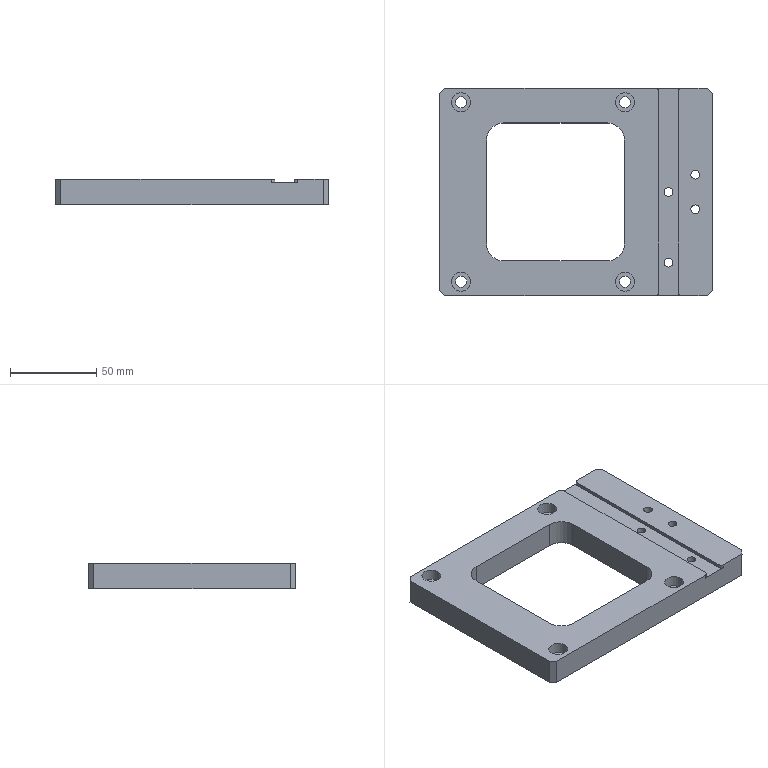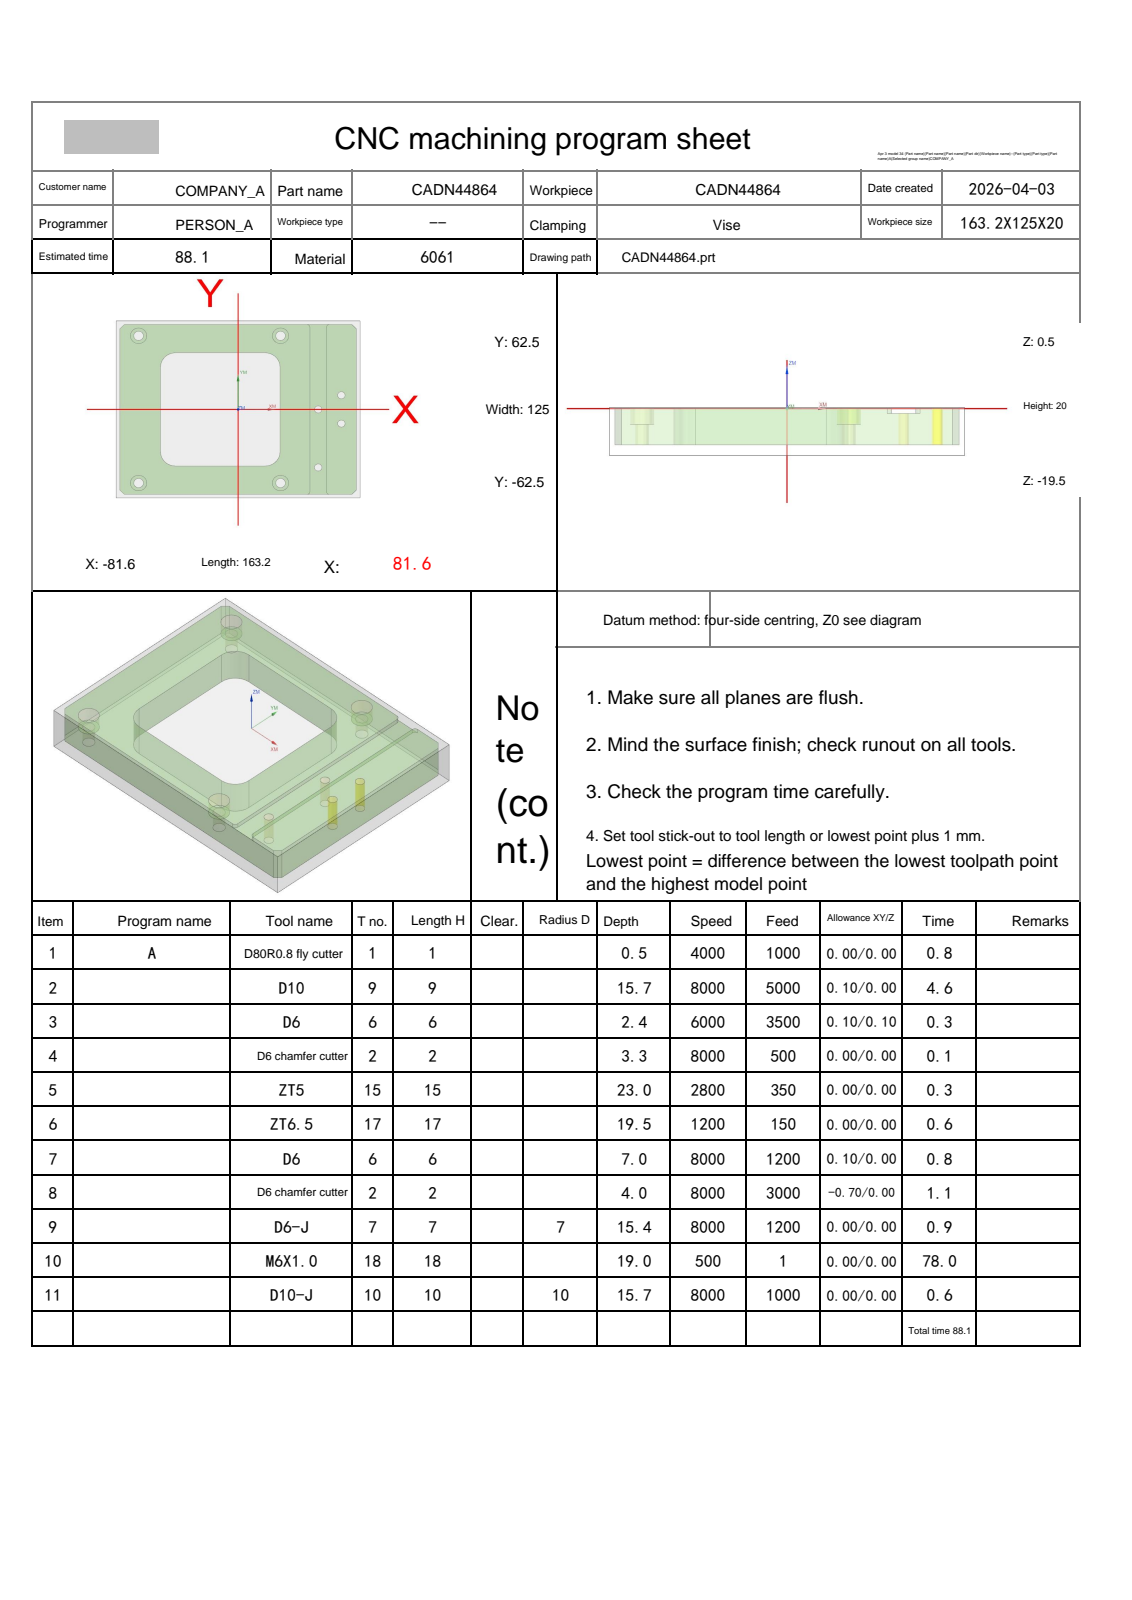NC program | NX | posted by the shop | part box 158.2 x 120 x 15 mm
Lines 961 to 2334 of 2334:
N8 T02 M06
(D6 chamfer cutter  D=6. R=0. H=02 ce=0.00 di=0.00)
G00 G90 G54 X57.022 Y-.25 M03 S8000
G43 H02 Z20.
M08
Z2.099
G01 Z-1.5 F3000.
G03 X57.322 Y-.33 I.3 J.52
X57.842 Y-.03 I0.0 J.6
G01 X57.85 Y0.0
Y58.
G02 X61.15 Y61.3 I3.3 J0.0
G01 X76.1
X76.354 Y61.275
X76.597 Y61.201
X76.822 Y61.081
X77.019 Y60.919
X80.019 Y57.919
X80.181 Y57.722
X80.301 Y57.498
X80.375 Y57.254
X80.4 Y57.
Y-57.
X80.375 Y-57.254
X80.301 Y-57.497
X80.181 Y-57.722
X80.019 Y-57.919
X77.019 Y-60.919
X76.822 Y-61.081
X76.597 Y-61.201
X76.354 Y-61.275
X76.1 Y-61.3
X61.15
G02 X57.85 Y-58. I0.0 J3.3
G01 Y0.0
X57.842 Y.03
G03 X57.322 Y.33 I-.52 J-.3
X57.022 Y.25 I0.0 J-.6
G01 Z2.099
G00 Z20.
X-15.275 Y62.128
Z2.099
G01 Z-1.5
G03 X-15.355 Y61.828 I.52 J-.3
X-15.055 Y61.308 I.6 J0.0
G01 X-15.025 Y61.3
X46.05
G02 X49.35 Y58. I0.0 J-3.3
G01 Y-58.
G02 X46.05 Y-61.3 I-3.3 J0.0
G01 X-76.1
X-76.353 Y-61.275
X-76.597 Y-61.201
X-76.822 Y-61.081
X-77.019 Y-60.919
X-80.019 Y-57.919
X-80.181 Y-57.722
X-80.301 Y-57.497
X-80.375 Y-57.254
X-80.4 Y-57.
Y57.
X-80.375 Y57.254
X-80.301 Y57.497
X-80.181 Y57.722
X-80.019 Y57.919
X-77.019 Y60.919
X-76.822 Y61.081
X-76.597 Y61.201
X-76.354 Y61.275
X-76.1 Y61.3
X-15.025
X-14.995 Y61.308
G03 X-14.695 Y61.828 I-.3 J.52
X-14.775 Y62.128 I-.6 J0.0
G01 Z2.099
G00 Z20.
X-11.65 Y37.872
Z2.099
G01 Z-1.5
G03 X-11.57 Y38.172 I-.52 J.3
X-11.87 Y38.692 I-.6 J0.0
G01 X-11.9 Y38.7
X-41.9
G03 X-50.6 Y30. I0.0 J-8.7
G01 Y-30.
G03 X-41.9 Y-38.7 I8.7 J0.0
G01 X18.1
G03 X26.8 Y-30. I0.0 J8.7
G01 Y30.
G03 X18.1 Y38.7 I-8.7 J0.0
G01 X-11.9
X-11.93 Y38.692
G03 X-12.23 Y38.172 I.3 J-.52
X-12.15 Y37.872 I.6 J0.0
G01 Z2.099
G00 Z20.
X56.976 Y-62.128
Z1.755
G01 Z-3.5
G03 X57.056 Y-61.828 I-.52 J.3
X56.756 Y-61.308 I-.6 J0.0
G01 X56.726 Y-61.3
X50.474
X50.444 Y-61.308
G03 X50.144 Y-61.828 I.3 J-.52
X50.224 Y-62.128 I.6 J0.0
G01 Z1.755
G00 Z20.
Y62.128
Z1.755
G01 Z-3.5
G03 X50.144 Y61.828 I.52 J-.3
X50.444 Y61.308 I.6 J0.0
G01 X50.474 Y61.3
X56.726
X56.756 Y61.308
G03 X57.056 Y61.828 I-.3 J.52
X56.976 Y62.128 I-.6 J0.0
G01 Z1.755
G00 Z20.
G00 G90 X69.257 Y9.216 M03 S8000
Z20.
Z-.5
G01 Z-1. F500.
X69.4 Y8.5
G03 X70.9 Y10. I0.0 J1.5
X69.1 Y11.8 I-1.8 J0.0
X67.3 Y10. I0.0 J-1.8
X69.1 Y8.2 I1.8 J0.0
X70.9 Y10. I0.0 J1.8
X69.4 Y11.5 I-1.5 J0.0
G01 X69.257 Y10.784
Z-.5
G00 Z20.
Y-10.784
Z-.5
G01 Z-1.
X69.4 Y-11.5
G03 X70.9 Y-10. I0.0 J1.5
X69.1 Y-8.2 I-1.8 J0.0
X67.3 Y-10. I0.0 J-1.8
X69.1 Y-11.8 I1.8 J0.0
X70.9 Y-10. I0.0 J1.8
X69.4 Y-8.5 I-1.5 J0.0
G01 X69.257 Y-9.216
Z-.5
G00 Z20.
G00 G90 X-68.609 Y47.643 M03 S8000
Z20.
Z2.5
G01 X-68.434 Y47.561 Z2.43 F800.
X-67.999 Y47.405 Z2.261
X-67.55 Y47.292 Z2.093
X-67.093 Y47.222 Z1.925
X-66.631 Y47.197 Z1.756
X-66.169 Y47.216 Z1.588
X-65.71 Y47.28 Z1.419
X-65.26 Y47.388 Z1.251
X-64.823 Y47.538 Z1.083
X-64.402 Y47.73 Z.914
X-64.001 Y47.961 Z.746
X-63.624 Y48.23 Z.577
X-63.275 Y48.534 Z.409
X-62.957 Y48.87 Z.241
X-62.673 Y49.235 Z.072
X-62.425 Y49.625 Z-.096
X-62.216 Y50.038 Z-.265
X-62.048 Y50.469 Z-.433
X-61.921 Y50.914 Z-.601
X-61.839 Y51.369 Z-.77
X-61.8 Y51.83 Z-.938
Y52. Z-1.
G03 X-66.6 Y56.8 I-4.8 J0.0
X-71.4 Y52. I0.0 J-4.8
X-66.6 Y47.2 I4.8 J0.0
X-61.8 Y52. I0.0 J4.8
X-61.826 Y52.499 I-4.8 J0.0
G01 Z1.5
G00 Z20.
X26.391 Y47.643
Z2.5
G01 X26.566 Y47.561 Z2.43
X27.001 Y47.405 Z2.261
X27.45 Y47.292 Z2.093
X27.907 Y47.222 Z1.925
X28.369 Y47.197 Z1.756
X28.831 Y47.216 Z1.588
X29.29 Y47.28 Z1.419
X29.74 Y47.388 Z1.251
X30.177 Y47.538 Z1.083
X30.598 Y47.73 Z.914
X30.999 Y47.961 Z.746
X31.376 Y48.23 Z.577
X31.725 Y48.534 Z.409
X32.043 Y48.87 Z.241
X32.327 Y49.235 Z.072
X32.575 Y49.625 Z-.096
X32.784 Y50.038 Z-.265
X32.952 Y50.469 Z-.433
X33.079 Y50.914 Z-.601
X33.161 Y51.369 Z-.77
X33.2 Y51.83 Z-.938
Y52. Z-1.
G03 X28.4 Y56.8 I-4.8 J0.0
X23.6 Y52. I0.0 J-4.8
X28.4 Y47.2 I4.8 J0.0
X33.2 Y52. I0.0 J4.8
X33.174 Y52.499 I-4.8 J0.0
G01 Z1.5
G00 Z20.
X26.391 Y-56.357
Z2.5
G01 X26.566 Y-56.439 Z2.43
X27.001 Y-56.595 Z2.261
X27.45 Y-56.708 Z2.093
X27.907 Y-56.778 Z1.925
X28.369 Y-56.803 Z1.756
X28.831 Y-56.784 Z1.588
X29.29 Y-56.72 Z1.419
X29.74 Y-56.612 Z1.251
X30.177 Y-56.462 Z1.083
X30.598 Y-56.27 Z.914
X30.999 Y-56.039 Z.746
X31.376 Y-55.77 Z.577
X31.725 Y-55.466 Z.409
X32.043 Y-55.13 Z.241
X32.327 Y-54.765 Z.072
X32.575 Y-54.375 Z-.096
X32.784 Y-53.962 Z-.265
X32.952 Y-53.531 Z-.433
X33.079 Y-53.086 Z-.601
X33.161 Y-52.631 Z-.77
X33.2 Y-52.17 Z-.938
Y-52. Z-1.
G03 X28.4 Y-47.2 I-4.8 J0.0
X23.6 Y-52. I0.0 J-4.8
X28.4 Y-56.8 I4.8 J0.0
X33.2 Y-52. I0.0 J4.8
X33.174 Y-51.501 I-4.8 J0.0
G01 Z1.5
G00 Z20.
X-68.609 Y-56.357
Z2.5
G01 X-68.434 Y-56.439 Z2.43
X-67.999 Y-56.595 Z2.261
X-67.55 Y-56.708 Z2.093
X-67.093 Y-56.778 Z1.925
X-66.631 Y-56.803 Z1.756
X-66.169 Y-56.784 Z1.588
X-65.71 Y-56.72 Z1.419
X-65.26 Y-56.612 Z1.251
X-64.823 Y-56.462 Z1.083
X-64.402 Y-56.27 Z.914
X-64.001 Y-56.039 Z.746
X-63.624 Y-55.77 Z.577
X-63.275 Y-55.466 Z.409
X-62.957 Y-55.13 Z.241
X-62.673 Y-54.765 Z.072
X-62.425 Y-54.375 Z-.096
X-62.216 Y-53.962 Z-.265
X-62.048 Y-53.531 Z-.433
X-61.921 Y-53.086 Z-.601
X-61.839 Y-52.631 Z-.77
X-61.8 Y-52.17 Z-.938
Y-52. Z-1.
G03 X-66.6 Y-47.2 I-4.8 J0.0
X-71.4 Y-52. I0.0 J-4.8
X-66.6 Y-56.8 I4.8 J0.0
X-61.8 Y-52. I0.0 J4.8
X-61.826 Y-51.501 I-4.8 J0.0
G01 Z1.5
G00 Z20.
G00 G90 X53.4 Y-41.003 M03 S8000
Z20.
Z.5
G01 Y-41.045 Z.499 F500.
X53.461 Y-41.151 Z.494
X53.539 Y-41.196 Z.491
X53.65 Y-41.199 Z.487
X53.747 Y-41.143 Z.483
X53.8 Y-41.045 Z.479
Y-40.955 Z.476
X53.747 Y-40.857 Z.472
X53.65 Y-40.801 Z.469
X53.539 Y-40.804 Z.465
X53.461 Y-40.849 Z.462
X53.4 Y-40.955 Z.457
Y-41.045 Z.454
X53.461 Y-41.151 Z.45
X53.539 Y-41.196 Z.447
X53.65 Y-41.199 Z.443
X53.747 Y-41.143 Z.439
X53.8 Y-41.045 Z.435
Y-40.955 Z.432
X53.747 Y-40.857 Z.428
X53.65 Y-40.801 Z.424
X53.539 Y-40.804 Z.42
X53.461 Y-40.849 Z.417
X53.4 Y-40.955 Z.413
Y-41.045 Z.41
X53.461 Y-41.151 Z.405
X53.539 Y-41.196 Z.402
X53.65 Y-41.199 Z.398
X53.747 Y-41.143 Z.394
X53.8 Y-41.045 Z.391
Y-40.955 Z.387
X53.747 Y-40.857 Z.384
X53.65 Y-40.801 Z.38
X53.539 Y-40.804 Z.376
X53.461 Y-40.849 Z.373
X53.4 Y-40.955 Z.368
Y-41.045 Z.365
X53.461 Y-41.151 Z.361
X53.539 Y-41.196 Z.358
X53.65 Y-41.199 Z.354
X53.747 Y-41.143 Z.35
X53.8 Y-41.045 Z.346
Y-40.955 Z.343
X53.747 Y-40.857 Z.339
X53.65 Y-40.801 Z.335
X53.539 Y-40.804 Z.331
X53.461 Y-40.849 Z.328
X53.4 Y-40.955 Z.324
Y-41.045 Z.321
X53.461 Y-41.151 Z.317
X53.539 Y-41.196 Z.313
X53.65 Y-41.199 Z.309
X53.747 Y-41.143 Z.306
X53.8 Y-41.045 Z.302
Y-40.955 Z.299
X53.747 Y-40.857 Z.295
X53.65 Y-40.801 Z.291
X53.539 Y-40.804 Z.287
X53.461 Y-40.849 Z.284
X53.4 Y-40.955 Z.279
Y-41.045 Z.276
X53.461 Y-41.151 Z.272
X53.539 Y-41.196 Z.269
X53.65 Y-41.199 Z.265
X53.747 Y-41.143 Z.261
X53.8 Y-41.045 Z.257
Y-40.955 Z.254
X53.747 Y-40.857 Z.25
X53.65 Y-40.801 Z.246
X53.539 Y-40.804 Z.242
X53.461 Y-40.849 Z.239
X53.4 Y-40.955 Z.235
Y-41.045 Z.232
X53.461 Y-41.151 Z.228
X53.539 Y-41.196 Z.224
X53.65 Y-41.199 Z.221
X53.747 Y-41.143 Z.217
X53.8 Y-41.045 Z.213
Y-40.955 Z.21
X53.747 Y-40.857 Z.206
X53.65 Y-40.801 Z.202
X53.539 Y-40.804 Z.198
X53.461 Y-40.849 Z.195
X53.4 Y-40.955 Z.191
Y-41.045 Z.187
X53.461 Y-41.151 Z.183
X53.539 Y-41.196 Z.18
X53.65 Y-41.199 Z.176
X53.747 Y-41.143 Z.172
X53.8 Y-41.045 Z.168
Y-40.955 Z.165
X53.747 Y-40.857 Z.161
X53.65 Y-40.801 Z.157
X53.539 Y-40.804 Z.154
X53.461 Y-40.849 Z.15
X53.4 Y-40.955 Z.146
Y-41.045 Z.143
X53.461 Y-41.151 Z.139
X53.539 Y-41.196 Z.136
X53.65 Y-41.199 Z.132
X53.747 Y-41.143 Z.128
X53.8 Y-41.045 Z.124
Y-40.955 Z.121
X53.747 Y-40.857 Z.117
X53.65 Y-40.801 Z.113
X53.539 Y-40.804 Z.109
X53.461 Y-40.849 Z.106
X53.4 Y-40.955 Z.102
Y-41.045 Z.099
X53.461 Y-41.151 Z.094
X53.539 Y-41.196 Z.091
X53.65 Y-41.199 Z.087
X53.747 Y-41.143 Z.083
X53.8 Y-41.045 Z.079
Y-40.955 Z.076
X53.747 Y-40.857 Z.072
X53.65 Y-40.801 Z.069
X53.539 Y-40.804 Z.065
X53.461 Y-40.849 Z.061
X53.4 Y-40.955 Z.057
Y-41.045 Z.054
X53.461 Y-41.151 Z.05
X53.539 Y-41.196 Z.047
X53.65 Y-41.199 Z.043
X53.747 Y-41.143 Z.039
X53.8 Y-41.045 Z.035
Y-40.955 Z.032
X53.747 Y-40.857 Z.028
X53.65 Y-40.801 Z.024
X53.539 Y-40.804 Z.02
X53.461 Y-40.849 Z.017
X53.4 Y-40.955 Z.013
Y-41.045 Z.01
X53.461 Y-41.151 Z.005
X53.539 Y-41.196 Z.002
X53.65 Y-41.199 Z-.002
X53.747 Y-41.143 Z-.006
X53.8 Y-41.045 Z-.009
Y-40.955 Z-.013
X53.747 Y-40.857 Z-.016
X53.65 Y-40.801 Z-.02
X53.539 Y-40.804 Z-.024
X53.461 Y-40.849 Z-.027
X53.4 Y-40.955 Z-.032
Y-41.045 Z-.035
X53.461 Y-41.151 Z-.039
X53.539 Y-41.196 Z-.042
X53.65 Y-41.199 Z-.046
X53.747 Y-41.143 Z-.05
X53.8 Y-41.045 Z-.054
Y-40.955 Z-.057
X53.747 Y-40.857 Z-.061
X53.65 Y-40.801 Z-.065
X53.539 Y-40.804 Z-.069
X53.461 Y-40.849 Z-.072
X53.4 Y-40.955 Z-.076
Y-41.045 Z-.079
X53.461 Y-41.151 Z-.084
X53.539 Y-41.196 Z-.087
X53.65 Y-41.199 Z-.091
X53.747 Y-41.143 Z-.094
X53.8 Y-41.045 Z-.098
Y-40.955 Z-.101
X53.747 Y-40.857 Z-.105
X53.65 Y-40.801 Z-.109
X53.539 Y-40.804 Z-.113
X53.461 Y-40.849 Z-.116
X53.4 Y-40.955 Z-.121
Y-41.045 Z-.124
X53.461 Y-41.151 Z-.128
X53.539 Y-41.196 Z-.131
X53.65 Y-41.199 Z-.135
X53.747 Y-41.143 Z-.139
X53.8 Y-41.045 Z-.143
Y-40.955 Z-.146
X53.747 Y-40.857 Z-.15
X53.65 Y-40.801 Z-.154
X53.539 Y-40.804 Z-.158
X53.461 Y-40.849 Z-.161
X53.4 Y-40.955 Z-.165
Y-41.045 Z-.168
X53.461 Y-41.151 Z-.172
X53.539 Y-41.196 Z-.176
X53.65 Y-41.199 Z-.179
X53.747 Y-41.143 Z-.183
X53.8 Y-41.045 Z-.187
Y-40.955 Z-.19
X53.747 Y-40.857 Z-.194
X53.65 Y-40.801 Z-.198
X53.539 Y-40.804 Z-.202
X53.461 Y-40.849 Z-.205
X53.4 Y-40.955 Z-.209
Y-41.045 Z-.213
X53.461 Y-41.151 Z-.217
X53.539 Y-41.196 Z-.22
X53.65 Y-41.199 Z-.224
X53.747 Y-41.143 Z-.228
X53.8 Y-41.045 Z-.232
Y-40.955 Z-.235
X53.747 Y-40.857 Z-.239
X53.65 Y-40.801 Z-.243
X53.539 Y-40.804 Z-.247
X53.461 Y-40.849 Z-.25
X53.4 Y-40.955 Z-.254
Y-41.045 Z-.257
X53.461 Y-41.151 Z-.261
X53.539 Y-41.196 Z-.264
X53.65 Y-41.199 Z-.268
X53.747 Y-41.143 Z-.272
X53.8 Y-41.045 Z-.276
Y-40.955 Z-.279
X53.747 Y-40.857 Z-.283
X53.65 Y-40.801 Z-.287
X53.539 Y-40.804 Z-.291
X53.461 Y-40.849 Z-.294
X53.4 Y-40.955 Z-.298
Y-41.045 Z-.302
X53.461 Y-41.151 Z-.306
X53.539 Y-41.196 Z-.309
X53.65 Y-41.199 Z-.313
X53.747 Y-41.143 Z-.317
X53.8 Y-41.045 Z-.321
Y-40.955 Z-.324
X53.747 Y-40.857 Z-.328
X53.65 Y-40.801 Z-.332
X53.539 Y-40.804 Z-.335
X53.461 Y-40.849 Z-.339
X53.4 Y-40.955 Z-.343
Y-41.045 Z-.346
X53.461 Y-41.151 Z-.35
X53.539 Y-41.196 Z-.353
X53.65 Y-41.199 Z-.357
X53.747 Y-41.143 Z-.361
X53.8 Y-41.045 Z-.365
Y-40.955 Z-.368
X53.747 Y-40.857 Z-.372
X53.65 Y-40.801 Z-.376
X53.539 Y-40.804 Z-.38
X53.461 Y-40.849 Z-.383
X53.4 Y-40.955 Z-.387
Y-41.045 Z-.39
X53.461 Y-41.151 Z-.395
X53.539 Y-41.196 Z-.398
X53.65 Y-41.199 Z-.402
X53.747 Y-41.143 Z-.406
X53.8 Y-41.045 Z-.409
Y-40.955 Z-.413
X53.747 Y-40.857 Z-.417
X53.65 Y-40.801 Z-.42
X53.539 Y-40.804 Z-.424
X53.461 Y-40.849 Z-.427
X53.4 Y-40.955 Z-.432
Y-41.045 Z-.435
X53.461 Y-41.151 Z-.439
X53.539 Y-41.196 Z-.442
X53.65 Y-41.199 Z-.446
X53.747 Y-41.143 Z-.45
X53.8 Y-41.045 Z-.454
Y-40.955 Z-.457
X53.747 Y-40.857 Z-.461
X53.65 Y-40.801 Z-.465
X53.539 Y-40.804 Z-.469
X53.461 Y-40.849 Z-.472
X53.4 Y-40.955 Z-.476
Y-41.045 Z-.479
X53.461 Y-41.151 Z-.484
X53.539 Y-41.196 Z-.487
X53.65 Y-41.199 Z-.491
X53.747 Y-41.143 Z-.494
X53.8 Y-41.045 Z-.498
Y-40.955 Z-.502
X53.747 Y-40.857 Z-.505
X53.65 Y-40.801 Z-.509
X53.539 Y-40.804 Z-.513
X53.461 Y-40.849 Z-.516
X53.4 Y-40.955 Z-.521
Y-41.045 Z-.524
X53.461 Y-41.151 Z-.528
X53.539 Y-41.196 Z-.531
X53.65 Y-41.199 Z-.535
X53.747 Y-41.143 Z-.539
X53.8 Y-41.045 Z-.543
Y-40.955 Z-.546
X53.747 Y-40.857 Z-.55
X53.65 Y-40.801 Z-.554
X53.539 Y-40.804 Z-.558
X53.461 Y-40.849 Z-.561
X53.4 Y-40.955 Z-.565
Y-41.045 Z-.568
X53.461 Y-41.151 Z-.572
X53.539 Y-41.196 Z-.576
X53.65 Y-41.199 Z-.579
X53.747 Y-41.143 Z-.583
X53.8 Y-41.045 Z-.587
Y-40.955 Z-.59
X53.747 Y-40.857 Z-.594
X53.65 Y-40.801 Z-.598
X53.539 Y-40.804 Z-.602
X53.461 Y-40.849 Z-.605
X53.4 Y-40.955 Z-.609
Y-41.045 Z-.613
X53.461 Y-41.151 Z-.617
X53.539 Y-41.196 Z-.62
X53.65 Y-41.199 Z-.624
X53.747 Y-41.143 Z-.628
X53.8 Y-41.045 Z-.632
Y-40.955 Z-.635
X53.747 Y-40.857 Z-.639
X53.65 Y-40.801 Z-.643
X53.539 Y-40.804 Z-.647
X53.461 Y-40.849 Z-.65
X53.4 Y-40.955 Z-.654
Y-41.045 Z-.657
X53.461 Y-41.151 Z-.661
X53.539 Y-41.196 Z-.664
X53.65 Y-41.199 Z-.668
X53.747 Y-41.143 Z-.672
X53.8 Y-41.045 Z-.676
Y-40.955 Z-.679
X53.747 Y-40.857 Z-.683
X53.65 Y-40.801 Z-.687
X53.539 Y-40.804 Z-.691
X53.461 Y-40.849 Z-.694
X53.4 Y-40.955 Z-.698
Y-41.045 Z-.702
X53.461 Y-41.151 Z-.706
X53.539 Y-41.196 Z-.709
X53.65 Y-41.199 Z-.713
X53.747 Y-41.143 Z-.717
X53.8 Y-41.045 Z-.721
Y-40.955 Z-.724
X53.747 Y-40.857 Z-.728
X53.65 Y-40.801 Z-.732
X53.539 Y-40.804 Z-.735
X53.461 Y-40.849 Z-.739
X53.4 Y-40.955 Z-.743
Y-41.045 Z-.746
X53.461 Y-41.151 Z-.75
X53.539 Y-41.196 Z-.753
X53.65 Y-41.199 Z-.757
X53.747 Y-41.143 Z-.761
X53.8 Y-41.045 Z-.765
Y-40.955 Z-.768
X53.747 Y-40.857 Z-.772
X53.65 Y-40.801 Z-.776
X53.539 Y-40.804 Z-.78
X53.461 Y-40.849 Z-.783
X53.4 Y-40.955 Z-.787
Y-41.045 Z-.79
X53.461 Y-41.151 Z-.795
X53.539 Y-41.196 Z-.798
X53.65 Y-41.199 Z-.802
X53.747 Y-41.143 Z-.806
X53.8 Y-41.045 Z-.81
Y-40.955 Z-.813
X53.747 Y-40.857 Z-.817
X53.65 Y-40.801 Z-.82
X53.539 Y-40.804 Z-.824
X53.461 Y-40.849 Z-.827
X53.4 Y-40.955 Z-.832
Y-41.045 Z-.835
X53.461 Y-41.151 Z-.839
X53.539 Y-41.196 Z-.842
X53.65 Y-41.199 Z-.846
X53.747 Y-41.143 Z-.85
X53.8 Y-41.045 Z-.854
Y-40.955 Z-.857
X53.747 Y-40.857 Z-.861
X53.65 Y-40.801 Z-.865
X53.539 Y-40.804 Z-.869
X53.461 Y-40.849 Z-.872
X53.4 Y-40.955 Z-.876
Y-41.045 Z-.879
X53.461 Y-41.151 Z-.884
X53.539 Y-41.196 Z-.887
X53.65 Y-41.199 Z-.891
X53.747 Y-41.143 Z-.895
X53.8 Y-41.045 Z-.898
Y-40.955 Z-.902
X53.747 Y-40.857 Z-.905
X53.65 Y-40.801 Z-.909
X53.539 Y-40.804 Z-.913
X53.461 Y-40.849 Z-.916
X53.4 Y-40.955 Z-.921
Y-41.045 Z-.924
X53.461 Y-41.151 Z-.928
X53.539 Y-41.196 Z-.931
X53.65 Y-41.199 Z-.935
X53.747 Y-41.143 Z-.939
X53.8 Y-41.045 Z-.943
Y-40.955 Z-.946
X53.747 Y-40.857 Z-.95
X53.65 Y-40.801 Z-.954
X53.539 Y-40.804 Z-.958
X53.461 Y-40.849 Z-.961
X53.4 Y-40.955 Z-.965
Y-41.045 Z-.968
X53.461 Y-41.151 Z-.972
X53.539 Y-41.196 Z-.976
X53.65 Y-41.199 Z-.98
X53.747 Y-41.143 Z-.983
X53.8 Y-41.045 Z-.987
Y-40.955 Z-.99
X53.747 Y-40.857 Z-.994
X53.65 Y-40.801 Z-.998
X53.539 Y-40.804 Z-1.002
X53.461 Y-40.849 Z-1.005
X53.4 Y-40.955 Z-1.01
Y-41.045 Z-1.013
X53.461 Y-41.151 Z-1.017
X53.539 Y-41.196 Z-1.02
X53.65 Y-41.199 Z-1.024
X53.747 Y-41.143 Z-1.028
X53.8 Y-41.045 Z-1.032
Y-40.955 Z-1.035
X53.747 Y-40.857 Z-1.039
X53.65 Y-40.801 Z-1.043
X53.539 Y-40.804 Z-1.047
X53.461 Y-40.849 Z-1.05
X53.4 Y-40.955 Z-1.054
Y-41.045 Z-1.057
X53.461 Y-41.151 Z-1.061
X53.539 Y-41.196 Z-1.065
X53.65 Y-41.199 Z-1.068
X53.747 Y-41.143 Z-1.072
X53.8 Y-41.045 Z-1.076
Y-40.955 Z-1.079
X53.747 Y-40.857 Z-1.083
X53.65 Y-40.801 Z-1.087
X53.539 Y-40.804 Z-1.091
X53.461 Y-40.849 Z-1.094
X53.4 Y-40.955 Z-1.098
Y-41. Z-1.1
G03 X53.6 Y-41.2 I.2 J0.0
X53.8 Y-41. I0.0 J.2
X53.6 Y-40.8 I-.2 J0.0
X53.4 Y-41. I0.0 J-.2
G01 Z-.6
G00 Z20.
X69.509 Y-11.021
Z-.6
G01 Z-1.1
X69.7 Y-11.5
G03 X71.2 Y-10. I0.0 J1.5
X69.1 Y-7.9 I-2.1 J0.0
X67. Y-10. I0.0 J-2.1
X69.1 Y-12.1 I2.1 J0.0
X71.2 Y-10. I0.0 J2.1
X69.7 Y-8.5 I-1.5 J0.0
G01 X69.509 Y-8.979
Z-.6
G00 Z20.
X53.4 Y-.003
Z.5
G01 Y-.045 Z.499
X53.461 Y-.151 Z.494
X53.539 Y-.196 Z.491
X53.65 Y-.199 Z.487
X53.747 Y-.143 Z.483
X53.8 Y-.045 Z.479
Y.045 Z.476
X53.747 Y.143 Z.472
X53.65 Y.199 Z.469
X53.539 Y.196 Z.465
X53.461 Y.151 Z.462
X53.4 Y.045 Z.457
Y-.045 Z.454
X53.461 Y-.151 Z.45
X53.539 Y-.196 Z.447
X53.65 Y-.199 Z.443
X53.747 Y-.143 Z.439
X53.8 Y-.045 Z.435
Y.045 Z.432
X53.747 Y.143 Z.428
X53.65 Y.199 Z.424
X53.539 Y.196 Z.42
X53.461 Y.151 Z.417
X53.4 Y.045 Z.413
Y-.045 Z.41
X53.461 Y-.151 Z.405
X53.539 Y-.196 Z.402
X53.65 Y-.199 Z.398
X53.747 Y-.143 Z.394
X53.8 Y-.045 Z.391
Y.045 Z.387
X53.747 Y.143 Z.384
X53.65 Y.199 Z.38
X53.539 Y.196 Z.376
X53.461 Y.151 Z.373
X53.4 Y.045 Z.368
Y-.045 Z.365
X53.461 Y-.151 Z.361
X53.539 Y-.196 Z.358
X53.65 Y-.199 Z.354
X53.747 Y-.143 Z.35
X53.8 Y-.045 Z.346
Y.045 Z.343
X53.747 Y.143 Z.339
X53.65 Y.199 Z.335
X53.539 Y.196 Z.331
X53.461 Y.151 Z.328
X53.4 Y.045 Z.324
Y-.045 Z.321
X53.461 Y-.151 Z.317
X53.539 Y-.196 Z.313
X53.65 Y-.199 Z.309
X53.747 Y-.143 Z.306
X53.8 Y-.045 Z.302
Y.045 Z.299
X53.747 Y.143 Z.295
X53.65 Y.199 Z.291
X53.539 Y.196 Z.287
X53.461 Y.151 Z.284
X53.4 Y.045 Z.279
Y-.045 Z.276
X53.461 Y-.151 Z.272
X53.539 Y-.196 Z.269
X53.65 Y-.199 Z.265
X53.747 Y-.143 Z.261
X53.8 Y-.045 Z.257
Y.045 Z.254
X53.747 Y.143 Z.25
X53.65 Y.199 Z.246
X53.539 Y.196 Z.242
X53.461 Y.151 Z.239
X53.4 Y.045 Z.235
Y-.045 Z.232
X53.461 Y-.151 Z.228
X53.539 Y-.196 Z.224
X53.65 Y-.199 Z.221
X53.747 Y-.143 Z.217
X53.8 Y-.045 Z.213
Y.045 Z.21
X53.747 Y.143 Z.206
X53.65 Y.199 Z.202
X53.539 Y.196 Z.198
X53.461 Y.151 Z.195
X53.4 Y.045 Z.191
Y-.045 Z.187
X53.461 Y-.151 Z.183
X53.539 Y-.196 Z.18
X53.65 Y-.199 Z.176
X53.747 Y-.143 Z.172
X53.8 Y-.045 Z.168
Y.045 Z.165
X53.747 Y.143 Z.161
X53.65 Y.199 Z.157
X53.539 Y.196 Z.154
X53.461 Y.151 Z.15
X53.4 Y.045 Z.146
Y-.045 Z.143
X53.461 Y-.151 Z.139
X53.539 Y-.196 Z.136
X53.65 Y-.199 Z.132
X53.747 Y-.143 Z.128
X53.8 Y-.045 Z.124
Y.045 Z.121
X53.747 Y.143 Z.117
X53.65 Y.199 Z.113
X53.539 Y.196 Z.109
X53.461 Y.151 Z.106
X53.4 Y.045 Z.102
Y-.045 Z.099
X53.461 Y-.151 Z.094
X53.539 Y-.196 Z.091
X53.65 Y-.199 Z.087
X53.747 Y-.143 Z.083
X53.8 Y-.045 Z.079
Y.045 Z.076
X53.747 Y.143 Z.072
X53.65 Y.199 Z.069
X53.539 Y.196 Z.065
X53.461 Y.151 Z.061
X53.4 Y.045 Z.057
Y-.045 Z.054
X53.461 Y-.151 Z.05
X53.539 Y-.196 Z.047
X53.65 Y-.199 Z.043
X53.747 Y-.143 Z.039
X53.8 Y-.045 Z.035
Y.045 Z.032
X53.747 Y.143 Z.028
X53.65 Y.199 Z.024
X53.539 Y.196 Z.02
X53.461 Y.151 Z.017
X53.4 Y.045 Z.013
Y-.045 Z.01
X53.461 Y-.151 Z.005
X53.539 Y-.196 Z.002
X53.65 Y-.199 Z-.002
X53.747 Y-.143 Z-.006
X53.8 Y-.045 Z-.009
Y.045 Z-.013
X53.747 Y.143 Z-.016
X53.65 Y.199 Z-.02
X53.539 Y.196 Z-.024
X53.461 Y.151 Z-.027
X53.4 Y.045 Z-.032
Y-.045 Z-.035
X53.461 Y-.151 Z-.039
X53.539 Y-.196 Z-.042
X53.65 Y-.199 Z-.046
X53.747 Y-.143 Z-.05
X53.8 Y-.045 Z-.054
Y.045 Z-.057
X53.747 Y.143 Z-.061
X53.65 Y.199 Z-.065
X53.539 Y.196 Z-.069
X53.461 Y.151 Z-.072
X53.4 Y.045 Z-.076
Y-.045 Z-.079
X53.461 Y-.151 Z-.084
X53.539 Y-.196 Z-.087
X53.65 Y-.199 Z-.091
X53.747 Y-.143 Z-.094
X53.8 Y-.045 Z-.098
Y.045 Z-.101
X53.747 Y.143 Z-.105
X53.65 Y.199 Z-.109
X53.539 Y.196 Z-.113
X53.461 Y.151 Z-.116
X53.4 Y.045 Z-.121
Y-.045 Z-.124
X53.461 Y-.151 Z-.128
X53.539 Y-.196 Z-.131
X53.65 Y-.199 Z-.135
X53.747 Y-.143 Z-.139
X53.8 Y-.045 Z-.143
Y.045 Z-.146
X53.747 Y.143 Z-.15
X53.65 Y.199 Z-.154
X53.539 Y.196 Z-.158
X53.461 Y.151 Z-.161
X53.4 Y.045 Z-.165
Y-.045 Z-.168
X53.461 Y-.151 Z-.172
X53.539 Y-.196 Z-.176
X53.65 Y-.199 Z-.179
X53.747 Y-.143 Z-.183
X53.8 Y-.045 Z-.187
Y.045 Z-.19
X53.747 Y.143 Z-.194
X53.65 Y.199 Z-.198
X53.539 Y.196 Z-.202
X53.461 Y.151 Z-.205
X53.4 Y.045 Z-.209
Y-.045 Z-.213
X53.461 Y-.151 Z-.217
X53.539 Y-.196 Z-.22
X53.65 Y-.199 Z-.224
X53.747 Y-.143 Z-.228
X53.8 Y-.045 Z-.232
Y.045 Z-.235
X53.747 Y.143 Z-.239
X53.65 Y.199 Z-.243
X53.539 Y.196 Z-.247
X53.461 Y.151 Z-.25
X53.4 Y.045 Z-.254
Y-.045 Z-.257
X53.461 Y-.151 Z-.261
X53.539 Y-.196 Z-.264
X53.65 Y-.199 Z-.268
X53.747 Y-.143 Z-.272
X53.8 Y-.045 Z-.276
Y.045 Z-.279
X53.747 Y.143 Z-.283
X53.65 Y.199 Z-.287
X53.539 Y.196 Z-.291
X53.461 Y.151 Z-.294
X53.4 Y.045 Z-.298
Y-.045 Z-.302
X53.461 Y-.151 Z-.306
X53.539 Y-.196 Z-.309
X53.65 Y-.199 Z-.313
X53.747 Y-.143 Z-.317
X53.8 Y-.045 Z-.321
Y.045 Z-.324
X53.747 Y.143 Z-.328
X53.65 Y.199 Z-.332
X53.539 Y.196 Z-.335
X53.461 Y.151 Z-.339
X53.4 Y.045 Z-.343
Y-.045 Z-.346
X53.461 Y-.151 Z-.35
X53.539 Y-.196 Z-.353
X53.65 Y-.199 Z-.357
X53.747 Y-.143 Z-.361
X53.8 Y-.045 Z-.365
Y.045 Z-.368
X53.747 Y.143 Z-.372
X53.65 Y.199 Z-.376
X53.539 Y.196 Z-.38
X53.461 Y.151 Z-.383
X53.4 Y.045 Z-.387
Y-.045 Z-.39
X53.461 Y-.151 Z-.395
X53.539 Y-.196 Z-.398
X53.65 Y-.199 Z-.402
X53.747 Y-.143 Z-.406
X53.8 Y-.045 Z-.409
Y.045 Z-.413
X53.747 Y.143 Z-.417
X53.65 Y.199 Z-.42
X53.539 Y.196 Z-.424
X53.461 Y.151 Z-.427
X53.4 Y.045 Z-.432
Y-.045 Z-.435
X53.461 Y-.151 Z-.439
X53.539 Y-.196 Z-.442
X53.65 Y-.199 Z-.446
X53.747 Y-.143 Z-.45
X53.8 Y-.045 Z-.454
Y.045 Z-.457
X53.747 Y.143 Z-.461
X53.65 Y.199 Z-.465
X53.539 Y.196 Z-.469
X53.461 Y.151 Z-.472
X53.4 Y.045 Z-.476
Y-.045 Z-.479
X53.461 Y-.151 Z-.484
X53.539 Y-.196 Z-.487
X53.65 Y-.199 Z-.491
X53.747 Y-.143 Z-.494
X53.8 Y-.045 Z-.498
Y.045 Z-.502
X53.747 Y.143 Z-.505
X53.65 Y.199 Z-.509
X53.539 Y.196 Z-.513
X53.461 Y.151 Z-.516
X53.4 Y.045 Z-.521
Y-.045 Z-.524
X53.461 Y-.151 Z-.528
X53.539 Y-.196 Z-.531
X53.65 Y-.199 Z-.535
X53.747 Y-.143 Z-.539
X53.8 Y-.045 Z-.543
Y.045 Z-.546
X53.747 Y.143 Z-.55
X53.65 Y.199 Z-.554
X53.539 Y.196 Z-.558
X53.461 Y.151 Z-.561
X53.4 Y.045 Z-.565
Y-.045 Z-.568
X53.461 Y-.151 Z-.572
X53.539 Y-.196 Z-.576
X53.65 Y-.199 Z-.579
X53.747 Y-.143 Z-.583
X53.8 Y-.045 Z-.587
Y.045 Z-.59
X53.747 Y.143 Z-.594
X53.65 Y.199 Z-.598
X53.539 Y.196 Z-.602
X53.461 Y.151 Z-.605
X53.4 Y.045 Z-.609
Y-.045 Z-.613
X53.461 Y-.151 Z-.617
X53.539 Y-.196 Z-.62
X53.65 Y-.199 Z-.624
X53.747 Y-.143 Z-.628
X53.8 Y-.045 Z-.632
Y.045 Z-.635
X53.747 Y.143 Z-.639
X53.65 Y.199 Z-.643
X53.539 Y.196 Z-.647
X53.461 Y.151 Z-.65
X53.4 Y.045 Z-.654
Y-.045 Z-.657
X53.461 Y-.151 Z-.661
X53.539 Y-.196 Z-.664
X53.65 Y-.199 Z-.668
X53.747 Y-.143 Z-.672
X53.8 Y-.045 Z-.676
Y.045 Z-.679
X53.747 Y.143 Z-.683
X53.65 Y.199 Z-.687
X53.539 Y.196 Z-.691
X53.461 Y.151 Z-.694
X53.4 Y.045 Z-.698
Y-.045 Z-.702
X53.461 Y-.151 Z-.706
X53.539 Y-.196 Z-.709
X53.65 Y-.199 Z-.713
X53.747 Y-.143 Z-.717
X53.8 Y-.045 Z-.721
Y.045 Z-.724
X53.747 Y.143 Z-.728
X53.65 Y.199 Z-.732
X53.539 Y.196 Z-.735
X53.461 Y.151 Z-.739
X53.4 Y.045 Z-.743
Y-.045 Z-.746
X53.461 Y-.151 Z-.75
X53.539 Y-.196 Z-.753
X53.65 Y-.199 Z-.757
X53.747 Y-.143 Z-.761
X53.8 Y-.045 Z-.765
Y.045 Z-.768
X53.747 Y.143 Z-.772
X53.65 Y.199 Z-.776
X53.539 Y.196 Z-.78
X53.461 Y.151 Z-.783
X53.4 Y.045 Z-.787
Y-.045 Z-.79
X53.461 Y-.151 Z-.795
X53.539 Y-.196 Z-.798
X53.65 Y-.199 Z-.802
X53.747 Y-.143 Z-.806
X53.8 Y-.045 Z-.81
Y.045 Z-.813
X53.747 Y.143 Z-.817
X53.65 Y.199 Z-.82
X53.539 Y.196 Z-.824
X53.461 Y.151 Z-.827
X53.4 Y.045 Z-.832
Y-.045 Z-.835
X53.461 Y-.151 Z-.839
X53.539 Y-.196 Z-.842
X53.65 Y-.199 Z-.846
X53.747 Y-.143 Z-.85
X53.8 Y-.045 Z-.854
Y.045 Z-.857
X53.747 Y.143 Z-.861
X53.65 Y.199 Z-.865
X53.539 Y.196 Z-.869
X53.461 Y.151 Z-.872
X53.4 Y.045 Z-.876
Y-.045 Z-.879
X53.461 Y-.151 Z-.884
X53.539 Y-.196 Z-.887
X53.65 Y-.199 Z-.891
X53.747 Y-.143 Z-.895
X53.8 Y-.045 Z-.898
Y.045 Z-.902
X53.747 Y.143 Z-.905
X53.65 Y.199 Z-.909
X53.539 Y.196 Z-.913
X53.461 Y.151 Z-.916
X53.4 Y.045 Z-.921
Y-.045 Z-.924
X53.461 Y-.151 Z-.928
X53.539 Y-.196 Z-.931
X53.65 Y-.199 Z-.935
X53.747 Y-.143 Z-.939
X53.8 Y-.045 Z-.943
Y.045 Z-.946
X53.747 Y.143 Z-.95
X53.65 Y.199 Z-.954
X53.539 Y.196 Z-.958
X53.461 Y.151 Z-.961
X53.4 Y.045 Z-.965
Y-.045 Z-.968
X53.461 Y-.151 Z-.972
X53.539 Y-.196 Z-.976
X53.65 Y-.199 Z-.98
X53.747 Y-.143 Z-.983
X53.8 Y-.045 Z-.987
Y.045 Z-.99
X53.747 Y.143 Z-.994
X53.65 Y.199 Z-.998
X53.539 Y.196 Z-1.002
X53.461 Y.151 Z-1.005
X53.4 Y.045 Z-1.01
Y-.045 Z-1.013
X53.461 Y-.151 Z-1.017
X53.539 Y-.196 Z-1.02
X53.65 Y-.199 Z-1.024
X53.747 Y-.143 Z-1.028
X53.8 Y-.045 Z-1.032
Y.045 Z-1.035
X53.747 Y.143 Z-1.039
X53.65 Y.199 Z-1.043
X53.539 Y.196 Z-1.047
X53.461 Y.151 Z-1.05
X53.4 Y.045 Z-1.054
Y-.045 Z-1.057
X53.461 Y-.151 Z-1.061
X53.539 Y-.196 Z-1.065
X53.65 Y-.199 Z-1.068
X53.747 Y-.143 Z-1.072
X53.8 Y-.045 Z-1.076
Y.045 Z-1.079
X53.747 Y.143 Z-1.083
X53.65 Y.199 Z-1.087
X53.539 Y.196 Z-1.091
X53.461 Y.151 Z-1.094
X53.4 Y.045 Z-1.098
Y0.0 Z-1.1
G03 X53.6 Y-.2 I.2 J0.0
X53.8 Y0.0 I0.0 J.2
X53.6 Y.2 I-.2 J0.0
X53.4 Y0.0 I0.0 J-.2
G01 Z-.6
G00 Z20.
X69.509 Y8.979
Z-.6
G01 Z-1.1
X69.7 Y8.5
G03 X71.2 Y10. I0.0 J1.5
X69.1 Y12.1 I-2.1 J0.0
X67. Y10. I0.0 J-2.1
X69.1 Y7.9 I2.1 J0.0
X71.2 Y10. I0.0 J2.1
X69.7 Y11.5 I-1.5 J0.0
G01 X69.509 Y11.021
Z-.6
G00 Z20.
G91 G28 Z0.0
M05
M09
G91 G28 Z0.0
M01
N9 T07 M06
(D6-J  D=6. R=0. H=07 ce=0.00 di=0.00)
G00 G90 G54 X28.4 Y52. M03 S8000
G43 H07 Z20.
M08
Z0.0
G41 D07
G01 X28.432 Y51.803 F500.
G03 X29.658 Y50.758 I1.226 J.197
X30.9 Y52. I0.0 J1.242
X30.9 Y52. Z-5. I-2.5 J0.0
X27.627 Y54.378 Z-6.5 I-2.5 J0.0
X25.9 Y52. I.773 J-2.378
X28.4 Y49.5 I2.5 J0.0
X30.9 Y52. I0.0 J2.5
X28.4 Y54.5 I-2.5 J0.0
X27.627 Y54.378 I0.0 J-2.5
X26.769 Y53.196 I.384 J-1.181
X28.011 Y51.954 I1.242 J0.0
G01 X28.202 Y51.969
G40 X28.4 Y52.
G00 Z20.
X-66.6
Z0.0
G41 D07
G01 X-66.568 Y51.803
G03 X-65.342 Y50.758 I1.226 J.197
X-64.1 Y52. I0.0 J1.242
X-64.1 Y52. Z-5. I-2.5 J0.0
X-67.373 Y54.378 Z-6.5 I-2.5 J0.0
X-69.1 Y52. I.773 J-2.378
X-66.6 Y49.5 I2.5 J0.0
X-64.1 Y52. I0.0 J2.5
X-66.6 Y54.5 I-2.5 J0.0
X-67.373 Y54.378 I0.0 J-2.5
X-68.231 Y53.196 I.384 J-1.181
X-66.989 Y51.954 I1.242 J0.0
G01 X-66.798 Y51.969
G40 X-66.6 Y52.
G00 Z20.
G00 G90 X28.4 Y-52. M03 S8000
Z20.
Z0.0
G41 D07
G01 X28.432 Y-52.197 F500.
G03 X29.658 Y-53.242 I1.226 J.197
X30.9 Y-52. I0.0 J1.242
X30.9 Y-52. Z-5. I-2.5 J0.0
X27.627 Y-49.622 Z-6.5 I-2.5 J0.0
X25.9 Y-52. I.773 J-2.378
X28.4 Y-54.5 I2.5 J0.0
X30.9 Y-52. I0.0 J2.5
X28.4 Y-49.5 I-2.5 J0.0
X27.627 Y-49.622 I0.0 J-2.5
X26.769 Y-50.804 I.384 J-1.181
X28.011 Y-52.046 I1.242 J0.0
G01 X28.202 Y-52.031
G40 X28.4 Y-52.
G00 Z20.
X-66.6
Z0.0
G41 D07
G01 X-66.568 Y-52.197
G03 X-65.342 Y-53.242 I1.226 J.197
X-64.1 Y-52. I0.0 J1.242
X-64.1 Y-52. Z-5. I-2.5 J0.0
X-67.373 Y-49.622 Z-6.5 I-2.5 J0.0
X-69.1 Y-52. I.773 J-2.378
X-66.6 Y-54.5 I2.5 J0.0
X-64.1 Y-52. I0.0 J2.5
X-66.6 Y-49.5 I-2.5 J0.0
X-67.373 Y-49.622 I0.0 J-2.5
X-68.231 Y-50.804 I.384 J-1.181
X-66.989 Y-52.046 I1.242 J0.0
G01 X-66.798 Y-52.031
G40 X-66.6 Y-52.
G00 Z20.
G00 G90 X64.85 Y-64.1 M03 S6000
Z20.
Z-1.5
G01 Z-2. F1200.
G41 D07
Y-64.
G03 X63.85 Y-63. I-1. J0.0
G01 X61.15
G02 X56.15 Y-58. I0.0 J5.
G01 Y58.
G02 X61.15 Y63. I5. J0.0
G01 X63.85
G03 X64.85 Y64. I0.0 J1.
G01 G40 Y64.1
Z-1.5
G00 Z20.
X42.35
Z-1.5
G01 Z-2.
G41 D07
Y64.
G03 X43.35 Y63. I1. J0.0
G01 X46.05
G02 X51.05 Y58. I0.0 J-5.
G01 Y-58.
G02 X46.05 Y-63. I-5. J0.0
G01 X43.35
G03 X42.35 Y-64. I0.0 J-1.
G01 G40 Y-64.1
Z-1.5
G00 Z20.
G00 G90 X-42.9 Y-35.816 M03 S6000
Z20.
Z-14.35
G01 Z-14.85 F1000.
G41 D07
Y-36.
G03 X-41.9 Y-37. I1. J0.0
G01 X18.1
G03 X25.1 Y-30. I0.0 J7.
G01 Y30.
G03 X18.1 Y37. I-7. J0.0
G01 X-41.9
G03 X-48.9 Y30. I0.0 J-7.
G01 Y-30.
G03 X-41.9 Y-37. I7. J0.0
G01 X-41.4
G03 X-40.4 Y-36. I0.0 J1.
G01 G40 Y-35.9
Z-14.35
G00 Z20.
G91 G28 Z0.0
M05
M09
G91 G28 Z0.0
M01
N10 T18 M06
(M6X1.0 D=5. DR_a=180 H=18)
G00 G90 G54 X53.6 Y-41. M03 S500
G43 H18 Z20.
M08
G95
G98 G84 X53.6 Y-41. Z-18.5 R1. F1. Q3.
X69.1 Y-10.
Y10.
X53.6 Y0.0
G80
G94
G00 Z20.
G91 G28 Z0.0
M05
M09
G91 G28 Z0.0
M01
N11 T10 M06
(D10-J  D=10. R=0. H=10 ce=0.00 di=0.00)
G00 G90 G54 X-77.113 Y66.116 M03 S8000
G43 H10 Z20.
M08
Z-14.7
G01 Z-15.2 F1000.
G41 D10
X-77.097 Y65.917
G03 X-76.1 Y65. I.997 J.083
G01 X76.1
G02 X79.636 Y63.536 I0.0 J-5.
G01 X82.636 Y60.536
G02 X84.1 Y57. I-3.536 J-3.536
G01 Y-57.
G02 X82.636 Y-60.536 I-5. J0.0
G01 X79.636 Y-63.536
G02 X76.1 Y-65. I-3.536 J3.536
G01 X-76.1
G02 X-79.636 Y-63.536 I0.0 J5.
G01 X-82.636 Y-60.536
G02 X-84.1 Y-57. I3.536 J3.536
G01 Y57.
G02 X-82.636 Y60.536 I5. J0.0
G01 X-79.636 Y63.536
G02 X-76.1 Y65. I3.536 J-3.536
G01 X-75.6
G03 X-74.6 Y66. I0.0 J1.
G01 G40 Y66.2
Z-14.7
G00 Z20.
M05
M09
G91 G28 Z0.0
G91 G28 Y0.0
M30
%